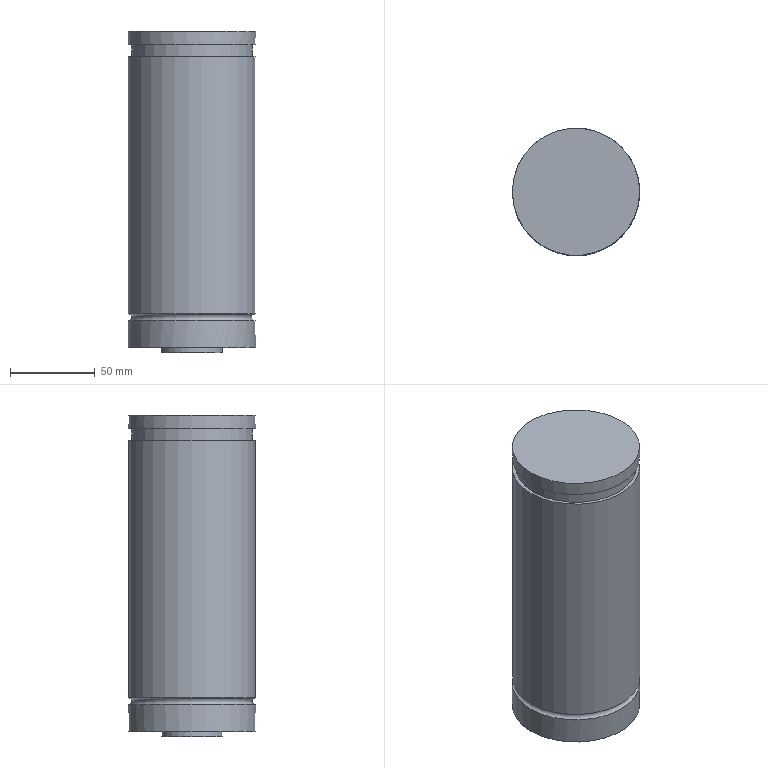Part | NX | features MAIN_BODY 2 | 1 solid | 11 faces | box 75.2 x 75.2 x 190 mm | volume 828936 mm3 | cylinder 5 | plane 5 | torus 1 | commonest cylinder face diameters 75.2 x3 36 x1 71.2 x1
STEP:
#1=CARTESIAN_POINT('',(-707.6,375.,375.));
#2=VERTEX_POINT('',#1);
#3=CARTESIAN_POINT('',(-670.,375.,375.));
#4=DIRECTION('',(0.,0.,-1.));
#5=DIRECTION('',(-1.,0.,0.));
#6=AXIS2_PLACEMENT_3D('',#3,#4,#5);
#7=CIRCLE('',#6,37.6);
#8=EDGE_CURVE('',#2,#2,#7,.F.);
#9=ORIENTED_EDGE('',*,*,#8,.F.);
#10=EDGE_LOOP('',(#9));
#11=FACE_BOUND('',#10,.T.);
#12=CARTESIAN_POINT('',(-707.6,375.,223.));
#13=VERTEX_POINT('',#12);
#14=CARTESIAN_POINT('',(-670.,375.,223.));
#15=DIRECTION('',(0.,0.,-1.));
#16=DIRECTION('',(-1.,0.,0.));
#17=AXIS2_PLACEMENT_3D('',#14,#15,#16);
#18=CIRCLE('',#17,37.6);
#19=EDGE_CURVE('',#13,#13,#18,.T.);
#20=ORIENTED_EDGE('',*,*,#19,.F.);
#21=EDGE_LOOP('',(#20));
#22=FACE_BOUND('',#21,.T.);
#23=CARTESIAN_POINT('',(-670.,375.,203.));
#24=DIRECTION('',(0.,0.,1.));
#25=DIRECTION('',(-1.,0.,0.));
#26=AXIS2_PLACEMENT_3D('',#23,#24,#25);
#27=CYLINDRICAL_SURFACE('',#26,37.6);
#28=ADVANCED_FACE('',(#11,#22),#27,.T.);
#29=CARTESIAN_POINT('',(-632.4,375.,203.));
#30=VERTEX_POINT('',#29);
#31=CARTESIAN_POINT('',(-670.,375.,203.));
#32=DIRECTION('',(0.,0.,1.));
#33=DIRECTION('',(1.,0.,0.));
#34=AXIS2_PLACEMENT_3D('',#31,#32,#33);
#35=CIRCLE('',#34,37.6);
#36=EDGE_CURVE('',#30,#30,#35,.T.);
#37=ORIENTED_EDGE('',*,*,#36,.F.);
#38=EDGE_LOOP('',(#37));
#39=FACE_BOUND('',#38,.T.);
#40=CARTESIAN_POINT('',(-652.,375.,203.));
#41=VERTEX_POINT('',#40);
#42=CARTESIAN_POINT('',(-670.,375.,203.));
#43=DIRECTION('',(0.,0.,1.));
#44=DIRECTION('',(1.,0.,0.));
#45=AXIS2_PLACEMENT_3D('',#42,#43,#44);
#46=CIRCLE('',#45,18.);
#47=EDGE_CURVE('',#41,#41,#46,.T.);
#48=ORIENTED_EDGE('',*,*,#47,.T.);
#49=EDGE_LOOP('',(#48));
#50=FACE_BOUND('',#49,.T.);
#51=CARTESIAN_POINT('',(-670.,375.,203.));
#52=DIRECTION('',(0.,0.,-1.));
#53=DIRECTION('',(1.,0.,0.));
#54=AXIS2_PLACEMENT_3D('',#51,#52,#53);
#55=PLANE('',#54);
#56=ADVANCED_FACE('',(#39,#50),#55,.T.);
#57=CARTESIAN_POINT('',(-707.6,375.,219.));
#58=VERTEX_POINT('',#57);
#59=CARTESIAN_POINT('',(-670.,375.,219.));
#60=DIRECTION('',(0.,0.,-1.));
#61=DIRECTION('',(-1.,0.,0.));
#62=AXIS2_PLACEMENT_3D('',#59,#60,#61);
#63=CIRCLE('',#62,37.6);
#64=EDGE_CURVE('',#58,#58,#63,.F.);
#65=ORIENTED_EDGE('',*,*,#64,.F.);
#66=EDGE_LOOP('',(#65));
#67=FACE_BOUND('',#66,.T.);
#68=ORIENTED_EDGE('',*,*,#36,.T.);
#69=EDGE_LOOP('',(#68));
#70=FACE_BOUND('',#69,.T.);
#71=CARTESIAN_POINT('',(-670.,375.,203.));
#72=DIRECTION('',(0.,0.,1.));
#73=DIRECTION('',(-1.,0.,0.));
#74=AXIS2_PLACEMENT_3D('',#71,#72,#73);
#75=CYLINDRICAL_SURFACE('',#74,37.6);
#76=ADVANCED_FACE('',(#67,#70),#75,.T.);
#77=CARTESIAN_POINT('',(-652.,375.,200.));
#78=VERTEX_POINT('',#77);
#79=CARTESIAN_POINT('',(-670.,375.,200.));
#80=DIRECTION('',(0.,0.,1.));
#81=DIRECTION('',(1.,0.,0.));
#82=AXIS2_PLACEMENT_3D('',#79,#80,#81);
#83=CIRCLE('',#82,18.);
#84=EDGE_CURVE('',#78,#78,#83,.T.);
#85=ORIENTED_EDGE('',*,*,#84,.T.);
#86=EDGE_LOOP('',(#85));
#87=FACE_BOUND('',#86,.T.);
#88=ORIENTED_EDGE('',*,*,#47,.F.);
#89=EDGE_LOOP('',(#88));
#90=FACE_BOUND('',#89,.T.);
#91=CARTESIAN_POINT('',(-670.,375.,200.));
#92=DIRECTION('',(0.,0.,1.));
#93=DIRECTION('',(-1.,0.,0.));
#94=AXIS2_PLACEMENT_3D('',#91,#92,#93);
#95=CYLINDRICAL_SURFACE('',#94,18.);
#96=ADVANCED_FACE('',(#87,#90),#95,.T.);
#97=ORIENTED_EDGE('',*,*,#84,.F.);
#98=EDGE_LOOP('',(#97));
#99=FACE_BOUND('',#98,.T.);
#100=CARTESIAN_POINT('',(-670.,375.,200.));
#101=DIRECTION('',(0.,0.,-1.));
#102=DIRECTION('',(1.,0.,0.));
#103=AXIS2_PLACEMENT_3D('',#100,#101,#102);
#104=PLANE('',#103);
#105=ADVANCED_FACE('',(#99),#104,.T.);
#106=ORIENTED_EDGE('',*,*,#64,.T.);
#107=EDGE_LOOP('',(#106));
#108=FACE_BOUND('',#107,.T.);
#109=ORIENTED_EDGE('',*,*,#19,.T.);
#110=EDGE_LOOP('',(#109));
#111=FACE_BOUND('',#110,.T.);
#112=CARTESIAN_POINT('',(-670.,375.,221.));
#113=DIRECTION('',(0.,0.,1.));
#114=DIRECTION('',(-1.,0.,0.));
#115=AXIS2_PLACEMENT_3D('',#112,#113,#114);
#116=TOROIDAL_SURFACE('',#115,37.6,2.);
#117=ADVANCED_FACE('',(#108,#111),#116,.F.);
#118=CARTESIAN_POINT('',(-634.4,375.,375.));
#119=VERTEX_POINT('',#118);
#120=CARTESIAN_POINT('',(-670.,375.,375.));
#121=DIRECTION('',(0.,0.,1.));
#122=DIRECTION('',(1.,0.,0.));
#123=AXIS2_PLACEMENT_3D('',#120,#121,#122);
#124=CIRCLE('',#123,35.6);
#125=EDGE_CURVE('',#119,#119,#124,.T.);
#126=ORIENTED_EDGE('',*,*,#125,.F.);
#127=EDGE_LOOP('',(#126));
#128=FACE_BOUND('',#127,.T.);
#129=ORIENTED_EDGE('',*,*,#8,.T.);
#130=EDGE_LOOP('',(#129));
#131=FACE_BOUND('',#130,.T.);
#132=CARTESIAN_POINT('',(-670.,375.,375.));
#133=DIRECTION('',(0.,0.,1.));
#134=DIRECTION('',(-1.,0.,0.));
#135=AXIS2_PLACEMENT_3D('',#132,#133,#134);
#136=PLANE('',#135);
#137=ADVANCED_FACE('',(#128,#131),#136,.T.);
#138=CARTESIAN_POINT('',(-634.4,375.,382.));
#139=VERTEX_POINT('',#138);
#140=CARTESIAN_POINT('',(-670.,375.,382.));
#141=DIRECTION('',(0.,0.,1.));
#142=DIRECTION('',(1.,0.,0.));
#143=AXIS2_PLACEMENT_3D('',#140,#141,#142);
#144=CIRCLE('',#143,35.6);
#145=EDGE_CURVE('',#139,#139,#144,.T.);
#146=ORIENTED_EDGE('',*,*,#145,.T.);
#147=EDGE_LOOP('',(#146));
#148=FACE_BOUND('',#147,.T.);
#149=CARTESIAN_POINT('',(-707.6,375.,382.));
#150=VERTEX_POINT('',#149);
#151=CARTESIAN_POINT('',(-670.,375.,382.));
#152=DIRECTION('',(0.,0.,-1.));
#153=DIRECTION('',(-1.,0.,0.));
#154=AXIS2_PLACEMENT_3D('',#151,#152,#153);
#155=CIRCLE('',#154,37.6);
#156=EDGE_CURVE('',#150,#150,#155,.T.);
#157=ORIENTED_EDGE('',*,*,#156,.T.);
#158=EDGE_LOOP('',(#157));
#159=FACE_BOUND('',#158,.T.);
#160=CARTESIAN_POINT('',(-670.,375.,382.));
#161=DIRECTION('',(0.,0.,1.));
#162=DIRECTION('',(-1.,0.,0.));
#163=AXIS2_PLACEMENT_3D('',#160,#161,#162);
#164=PLANE('',#163);
#165=ADVANCED_FACE('',(#148,#159),#164,.F.);
#166=ORIENTED_EDGE('',*,*,#125,.T.);
#167=EDGE_LOOP('',(#166));
#168=FACE_BOUND('',#167,.T.);
#169=ORIENTED_EDGE('',*,*,#145,.F.);
#170=EDGE_LOOP('',(#169));
#171=FACE_BOUND('',#170,.T.);
#172=CARTESIAN_POINT('',(-670.,375.,382.));
#173=DIRECTION('',(0.,0.,-1.));
#174=DIRECTION('',(1.,0.,0.));
#175=AXIS2_PLACEMENT_3D('',#172,#173,#174);
#176=CYLINDRICAL_SURFACE('',#175,35.6);
#177=ADVANCED_FACE('',(#168,#171),#176,.T.);
#178=CARTESIAN_POINT('',(-632.4,375.,390.));
#179=VERTEX_POINT('',#178);
#180=CARTESIAN_POINT('',(-670.,375.,390.));
#181=DIRECTION('',(0.,0.,1.));
#182=DIRECTION('',(1.,0.,0.));
#183=AXIS2_PLACEMENT_3D('',#180,#181,#182);
#184=CIRCLE('',#183,37.6);
#185=EDGE_CURVE('',#179,#179,#184,.T.);
#186=ORIENTED_EDGE('',*,*,#185,.T.);
#187=EDGE_LOOP('',(#186));
#188=FACE_BOUND('',#187,.T.);
#189=CARTESIAN_POINT('',(-670.,375.,390.));
#190=DIRECTION('',(0.,0.,-1.));
#191=DIRECTION('',(1.,0.,0.));
#192=AXIS2_PLACEMENT_3D('',#189,#190,#191);
#193=PLANE('',#192);
#194=ADVANCED_FACE('',(#188),#193,.F.);
#195=ORIENTED_EDGE('',*,*,#156,.F.);
#196=EDGE_LOOP('',(#195));
#197=FACE_BOUND('',#196,.T.);
#198=ORIENTED_EDGE('',*,*,#185,.F.);
#199=EDGE_LOOP('',(#198));
#200=FACE_BOUND('',#199,.T.);
#201=CARTESIAN_POINT('',(-670.,375.,203.));
#202=DIRECTION('',(0.,0.,1.));
#203=DIRECTION('',(-1.,0.,0.));
#204=AXIS2_PLACEMENT_3D('',#201,#202,#203);
#205=CYLINDRICAL_SURFACE('',#204,37.6);
#206=ADVANCED_FACE('',(#197,#200),#205,.T.);
#207=CLOSED_SHELL('',(#28,#56,#76,#96,#105,#117,#137,#165,#177,#194,#206));
#208=MANIFOLD_SOLID_BREP('',#207);
#209=(LENGTH_UNIT()NAMED_UNIT(*)SI_UNIT(.MILLI.,.METRE.));
#210=UNCERTAINTY_MEASURE_WITH_UNIT(LENGTH_MEASURE(0.00001),#209,'','');
#211=(NAMED_UNIT(*)PLANE_ANGLE_UNIT()SI_UNIT($,.RADIAN.));
#212=(NAMED_UNIT(*)SI_UNIT($,.STERADIAN.)SOLID_ANGLE_UNIT());
#213=(GEOMETRIC_REPRESENTATION_CONTEXT(3)GLOBAL_UNCERTAINTY_ASSIGNED_CONTEXT((#210))GLOBAL_UNIT_ASSIGNED_CONTEXT((#209,#211,#212))REPRESENTATION_CONTEXT('',''));
#214=ADVANCED_BREP_SHAPE_REPRESENTATION('',(#208),#213);